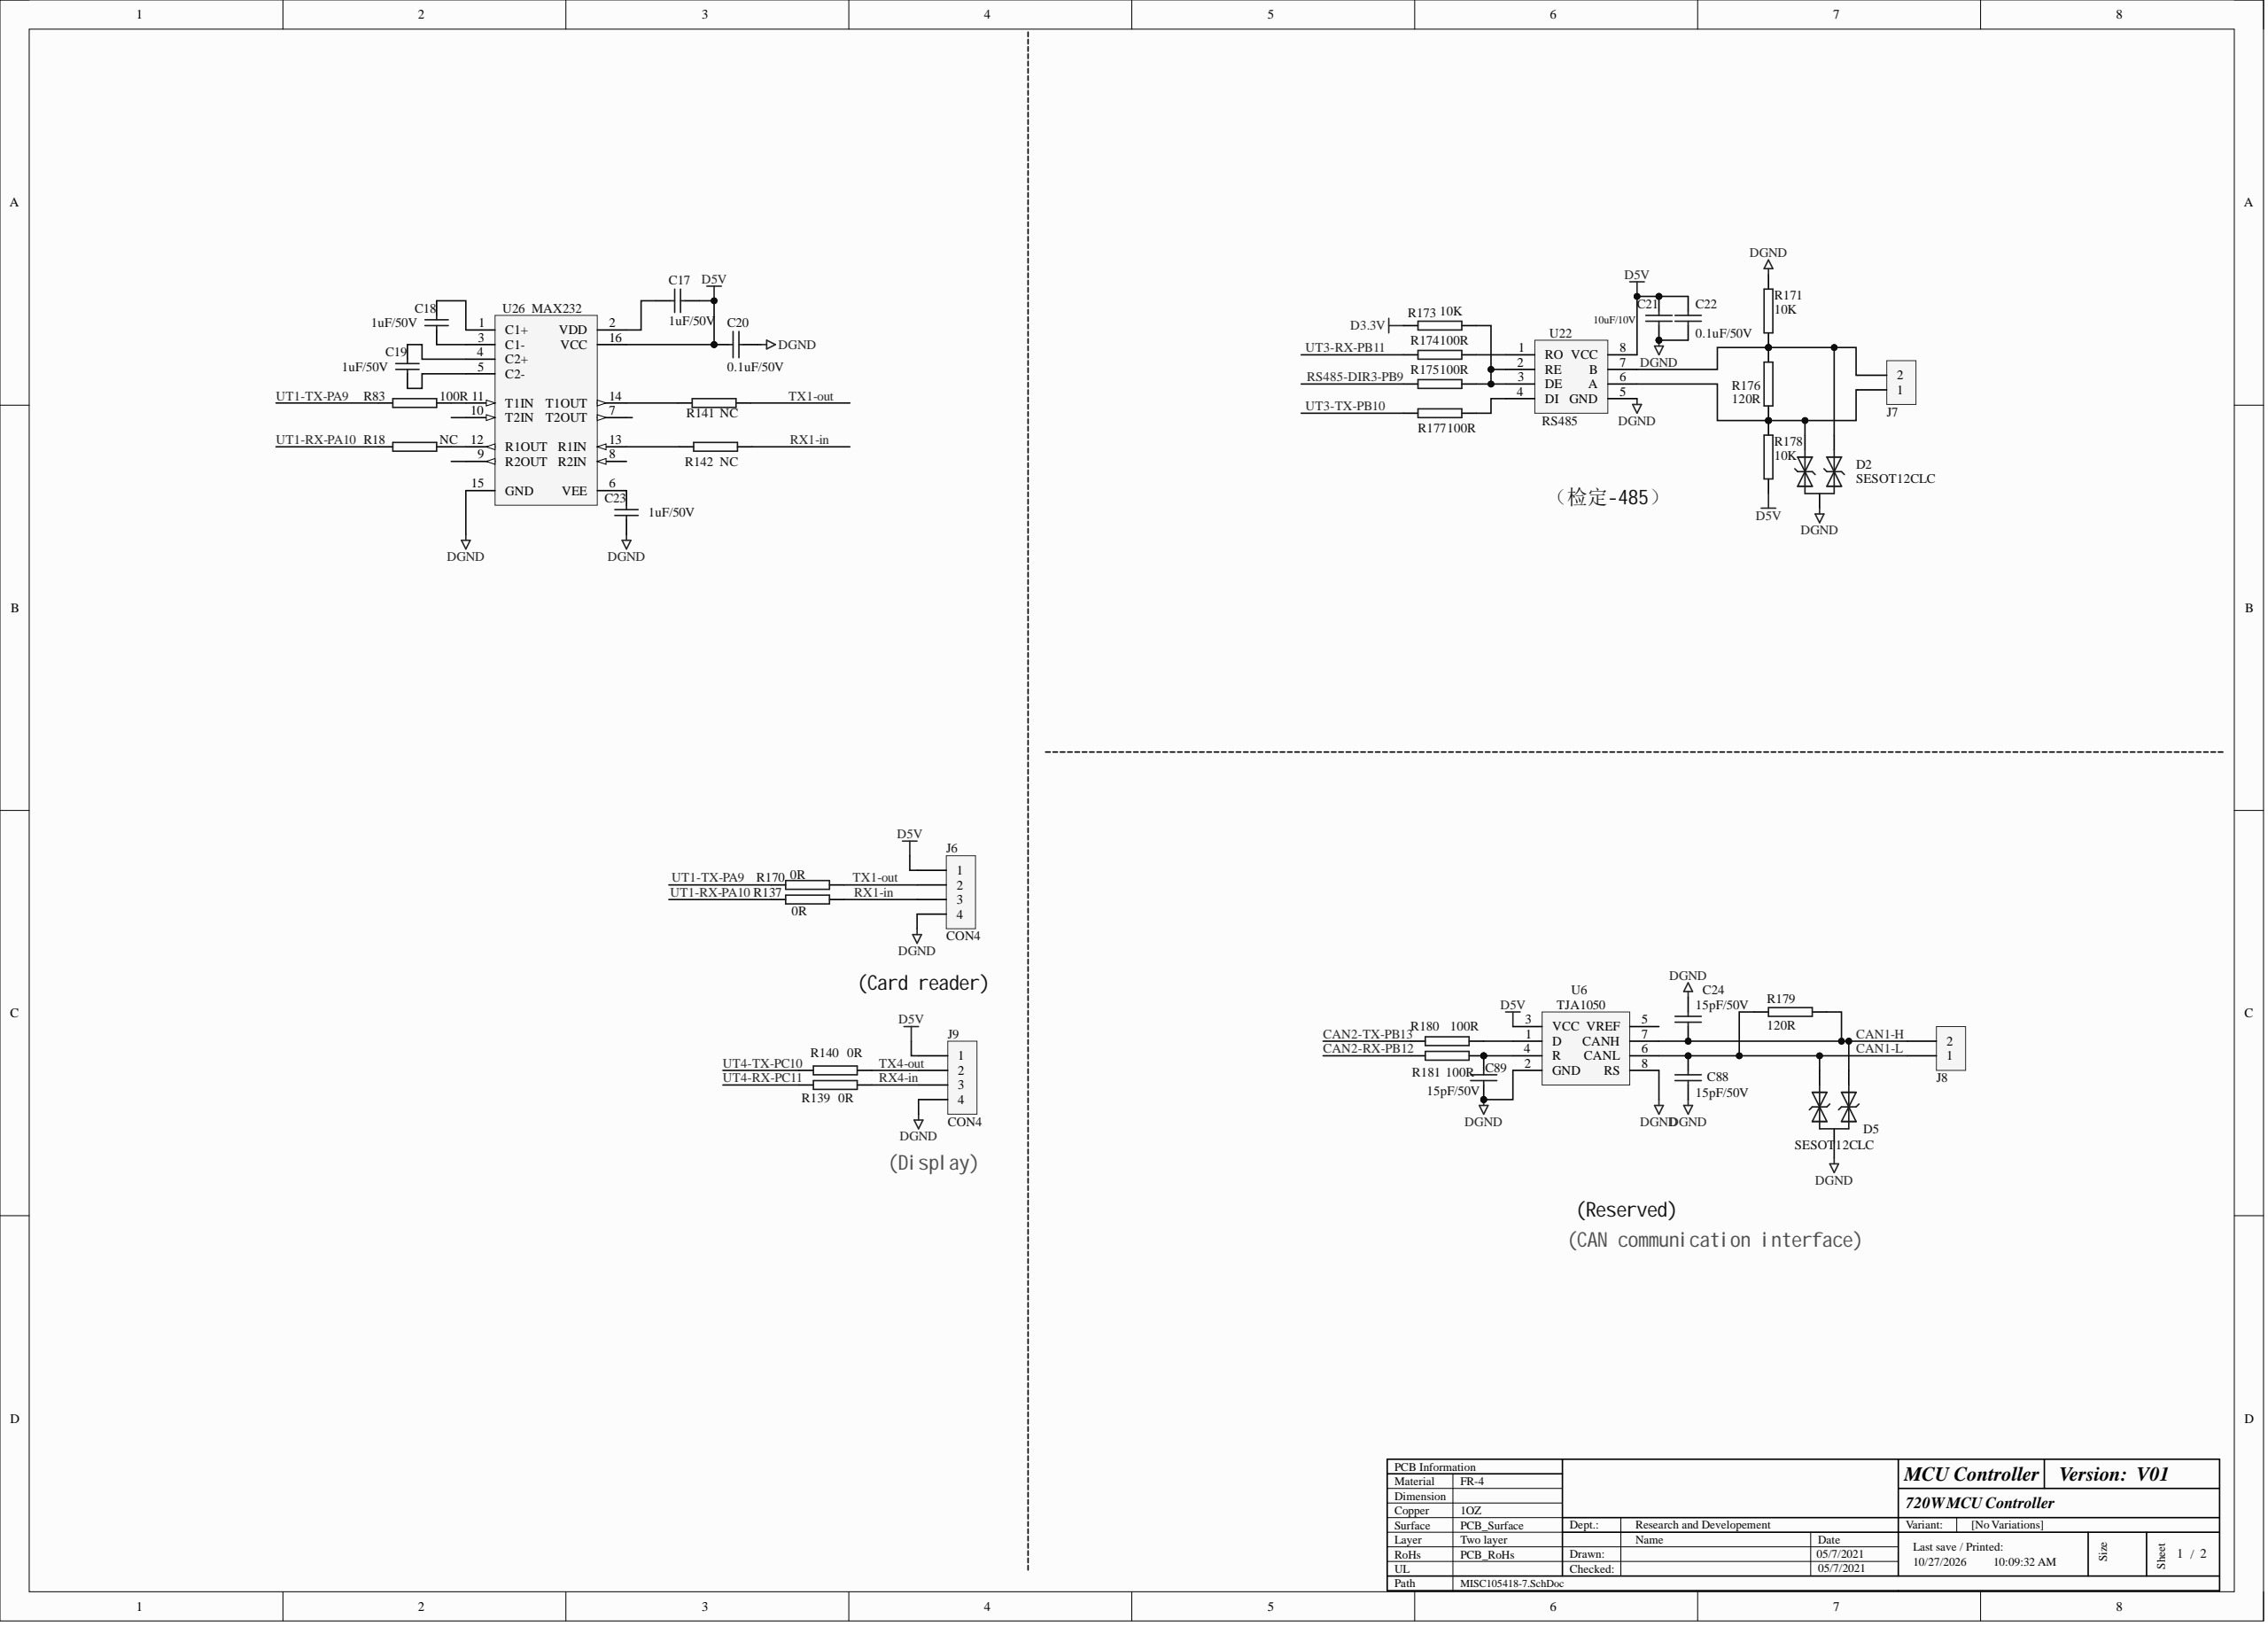Circuit board | Altium Designer | 455 parts | 280 nets | one sheet of the schematic
Parts on this sheet (reference | value | footprint):
C17 | 1uF/50V | CAP/0805
C18 | 1uF/50V | CAP/0805
C19 | 1uF/50V | CAP/0805
C20 | 0.1uF/50V | CAP/0603
C21 | 10uF/10V | C0805-T
C22 | 0.1uF/50V | C0603-T
C23 | 1uF/50V | CAP/0805
C24 | 15pF/50V | C0603-T
C88 | 15pF/50V | C0603-T
C89 | 15pF/50V | C0603-T
D2 | SESOT12CLC | SOT-23-T
D5 | SESOT12CLC | SOT-23-T
J6 | CON4 | CON4-2.5
J7 | CON2 | CON2-3.81
J8 | CON2 | CON2-3.81
J9 | CON4 | CON4-2.5
R18 | NC | RES/0603
R83 | 100R | RES/0603
R137 | 0R | R0603-T
R139 | 0R | R0805-T
R140 | 0R | R0805-T
R141 | NC | RES/0603
R142 | NC | RES/0603
R170 | 0R | R0603-T
R171 | 10K | R0603-T
R173 | 10K | R0603-T
R176 | 120R | R0805-T
R178 | 10K | R0603-T
R179 | 120R | R0805-T
R180 | 100R | R0603-T
R181 | 100R | R0603-T
U6 | TJA1050 | SO-8-T
U22 | RS485 | SO-8-T
U26 | MAX232 | SO-16-T
Nets of these parts (net: part-pin ...):
UT4-TX-PC10: R140-1
UT4-RX-PC11: R139-1
UT1-TX-PA9: R83-1 R170-1
UT1-RX-PA10: R18-1 R137-1
TX4-out: J9-2 R140-2
TX1-out: J6-2 R141-2 R170-2
RX4-in: J9-3 R139-2
RX1-in: J6-3 R137-2 R142-2
NetR180_1: R180-1 U6-1
NetR177_2: U22-4
NetR174_2: U22-1
NetR173_2: R173-2 U22-2 U22-3
NetR142_1: R142-1 U26-13
NetR141_1: R141-1 U26-14
NetR83_2: R83-2 U26-11
NetR18_2: R18-2 U26-12
NetD2_2: D2-2 J7-2 R171-1 R176-2 U22-7
NetD2_1: D2-1 J7-1 R176-1 R178-2 U22-6
NetC89_1: C89-1 R181-1 U6-4
NetC23_2: C23-2 U26-6
NetC19_2: C19-2 U26-4
NetC19_1: C19-1 U26-5
NetC18_2: C18-2 U26-1
NetC18_1: C18-1 U26-3
NetC17_2: C17-2 U26-2
D5V: C17-1 C20-1 C21-1 C22-1 J6-1 J9-1 R178-1 U6-3 U22-8 U26-16
D3.3V: R173-1
CAN2-TX-PB13: R180-2
CAN2-RX-PB12: R181-2
CAN1-L: C88-1 D5-2 J8-1 R179-2 U6-6
CAN1-H: C24-2 D5-1 J8-2 R179-1 U6-7
-: C20-2 C21-2 C22-2 C23-1 C24-1 C88-2 C89-2 D2-3 D5-3 J6-4 J9-4 R171-2 U6-2 U6-8 U22-5 U26-15